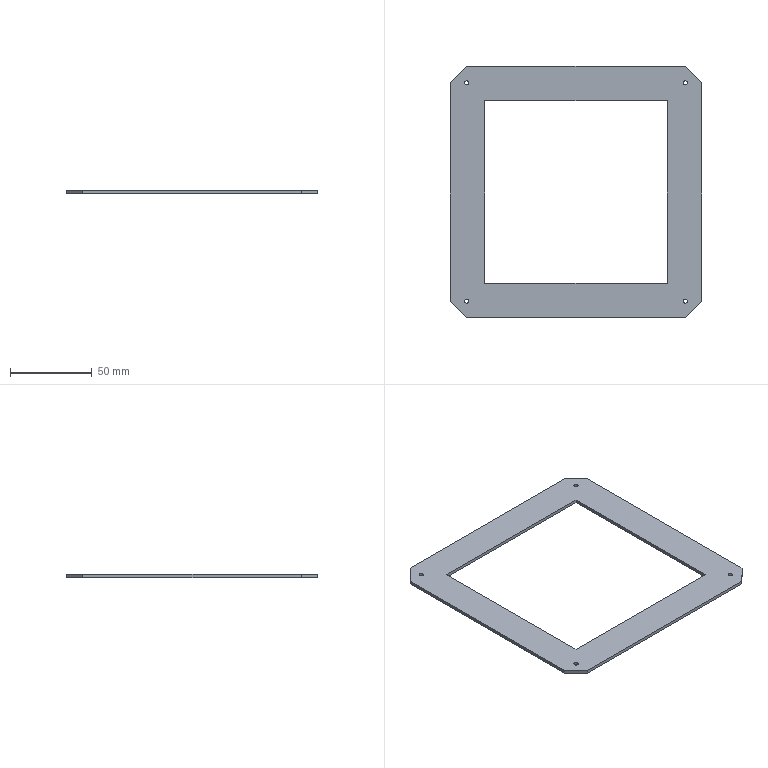Part | STEP file | 11-TG-00111 | 1 solid | 22 faces | box 154 x 154 x 2 mm | volume 21905 mm3 | plane 14 | cylinder 8 | commonest cylinder face diameters 2.5 x8
STEP:
#1=CARTESIAN_POINT('',(8.75,10.,0.));
#2=VERTEX_POINT('',#1);
#3=CARTESIAN_POINT('',(11.25,10.,0.));
#4=VERTEX_POINT('',#3);
#5=CARTESIAN_POINT('',(10.,10.,0.));
#6=DIRECTION('',(0.,0.,1.));
#7=DIRECTION('',(1.,0.,0.));
#8=AXIS2_PLACEMENT_3D('',#5,#6,#7);
#9=CIRCLE('',#8,1.25);
#10=EDGE_CURVE('',#2,#4,#9,.T.);
#11=ORIENTED_EDGE('',*,*,#10,.F.);
#12=CARTESIAN_POINT('',(8.75,10.,2.));
#13=VERTEX_POINT('',#12);
#14=CARTESIAN_POINT('',(8.75,10.,2.));
#15=DIRECTION('',(0.,0.,1.));
#16=VECTOR('',#15,1000.);
#17=LINE('',#14,#16);
#18=EDGE_CURVE('',#2,#13,#17,.T.);
#19=ORIENTED_EDGE('',*,*,#18,.T.);
#20=CARTESIAN_POINT('',(11.25,10.,2.));
#21=VERTEX_POINT('',#20);
#22=CARTESIAN_POINT('',(10.,10.,2.));
#23=DIRECTION('',(0.,0.,1.));
#24=DIRECTION('',(1.,0.,0.));
#25=AXIS2_PLACEMENT_3D('',#22,#23,#24);
#26=CIRCLE('',#25,1.25);
#27=EDGE_CURVE('',#13,#21,#26,.T.);
#28=ORIENTED_EDGE('',*,*,#27,.T.);
#29=CARTESIAN_POINT('',(11.25,10.,2.));
#30=DIRECTION('',(0.,0.,1.));
#31=VECTOR('',#30,1000.);
#32=LINE('',#29,#31);
#33=EDGE_CURVE('',#4,#21,#32,.T.);
#34=ORIENTED_EDGE('',*,*,#33,.F.);
#35=EDGE_LOOP('',(#11,#19,#28,#34));
#36=FACE_OUTER_BOUND('',#35,.T.);
#37=CARTESIAN_POINT('',(10.,10.,2.));
#38=DIRECTION('',(0.,0.,1.));
#39=DIRECTION('',(1.,0.,0.));
#40=AXIS2_PLACEMENT_3D('',#37,#38,#39);
#41=CYLINDRICAL_SURFACE('',#40,1.25);
#42=ADVANCED_FACE('',(#36),#41,.F.);
#43=CARTESIAN_POINT('',(142.75,10.,0.));
#44=VERTEX_POINT('',#43);
#45=CARTESIAN_POINT('',(145.25,10.,0.));
#46=VERTEX_POINT('',#45);
#47=CARTESIAN_POINT('',(144.,10.,0.));
#48=DIRECTION('',(0.,0.,1.));
#49=DIRECTION('',(1.,0.,0.));
#50=AXIS2_PLACEMENT_3D('',#47,#48,#49);
#51=CIRCLE('',#50,1.25);
#52=EDGE_CURVE('',#44,#46,#51,.T.);
#53=ORIENTED_EDGE('',*,*,#52,.F.);
#54=CARTESIAN_POINT('',(142.75,10.,2.));
#55=VERTEX_POINT('',#54);
#56=CARTESIAN_POINT('',(142.75,10.,2.));
#57=DIRECTION('',(0.,0.,1.));
#58=VECTOR('',#57,1000.);
#59=LINE('',#56,#58);
#60=EDGE_CURVE('',#44,#55,#59,.T.);
#61=ORIENTED_EDGE('',*,*,#60,.T.);
#62=CARTESIAN_POINT('',(145.25,10.,2.));
#63=VERTEX_POINT('',#62);
#64=CARTESIAN_POINT('',(144.,10.,2.));
#65=DIRECTION('',(0.,0.,1.));
#66=DIRECTION('',(1.,0.,0.));
#67=AXIS2_PLACEMENT_3D('',#64,#65,#66);
#68=CIRCLE('',#67,1.25);
#69=EDGE_CURVE('',#55,#63,#68,.T.);
#70=ORIENTED_EDGE('',*,*,#69,.T.);
#71=CARTESIAN_POINT('',(145.25,10.,2.));
#72=DIRECTION('',(0.,0.,1.));
#73=VECTOR('',#72,1000.);
#74=LINE('',#71,#73);
#75=EDGE_CURVE('',#46,#63,#74,.T.);
#76=ORIENTED_EDGE('',*,*,#75,.F.);
#77=EDGE_LOOP('',(#53,#61,#70,#76));
#78=FACE_OUTER_BOUND('',#77,.T.);
#79=CARTESIAN_POINT('',(144.,10.,2.));
#80=DIRECTION('',(0.,0.,1.));
#81=DIRECTION('',(1.,0.,0.));
#82=AXIS2_PLACEMENT_3D('',#79,#80,#81);
#83=CYLINDRICAL_SURFACE('',#82,1.25);
#84=ADVANCED_FACE('',(#78),#83,.F.);
#85=CARTESIAN_POINT('',(142.75,144.,0.));
#86=VERTEX_POINT('',#85);
#87=CARTESIAN_POINT('',(145.25,144.,0.));
#88=VERTEX_POINT('',#87);
#89=CARTESIAN_POINT('',(144.,144.,0.));
#90=DIRECTION('',(0.,0.,1.));
#91=DIRECTION('',(1.,0.,0.));
#92=AXIS2_PLACEMENT_3D('',#89,#90,#91);
#93=CIRCLE('',#92,1.25);
#94=EDGE_CURVE('',#86,#88,#93,.T.);
#95=ORIENTED_EDGE('',*,*,#94,.F.);
#96=CARTESIAN_POINT('',(142.75,144.,2.));
#97=VERTEX_POINT('',#96);
#98=CARTESIAN_POINT('',(142.75,144.,2.));
#99=DIRECTION('',(0.,0.,1.));
#100=VECTOR('',#99,1000.);
#101=LINE('',#98,#100);
#102=EDGE_CURVE('',#86,#97,#101,.T.);
#103=ORIENTED_EDGE('',*,*,#102,.T.);
#104=CARTESIAN_POINT('',(145.25,144.,2.));
#105=VERTEX_POINT('',#104);
#106=CARTESIAN_POINT('',(144.,144.,2.));
#107=DIRECTION('',(0.,0.,1.));
#108=DIRECTION('',(1.,0.,0.));
#109=AXIS2_PLACEMENT_3D('',#106,#107,#108);
#110=CIRCLE('',#109,1.25);
#111=EDGE_CURVE('',#97,#105,#110,.T.);
#112=ORIENTED_EDGE('',*,*,#111,.T.);
#113=CARTESIAN_POINT('',(145.25,144.,2.));
#114=DIRECTION('',(0.,0.,1.));
#115=VECTOR('',#114,1000.);
#116=LINE('',#113,#115);
#117=EDGE_CURVE('',#88,#105,#116,.T.);
#118=ORIENTED_EDGE('',*,*,#117,.F.);
#119=EDGE_LOOP('',(#95,#103,#112,#118));
#120=FACE_OUTER_BOUND('',#119,.T.);
#121=CARTESIAN_POINT('',(144.,144.,2.));
#122=DIRECTION('',(0.,0.,1.));
#123=DIRECTION('',(1.,0.,0.));
#124=AXIS2_PLACEMENT_3D('',#121,#122,#123);
#125=CYLINDRICAL_SURFACE('',#124,1.25);
#126=ADVANCED_FACE('',(#120),#125,.F.);
#127=CARTESIAN_POINT('',(8.75,144.,0.));
#128=VERTEX_POINT('',#127);
#129=CARTESIAN_POINT('',(11.25,144.,0.));
#130=VERTEX_POINT('',#129);
#131=CARTESIAN_POINT('',(10.,144.,0.));
#132=DIRECTION('',(0.,0.,1.));
#133=DIRECTION('',(1.,0.,0.));
#134=AXIS2_PLACEMENT_3D('',#131,#132,#133);
#135=CIRCLE('',#134,1.25);
#136=EDGE_CURVE('',#128,#130,#135,.T.);
#137=ORIENTED_EDGE('',*,*,#136,.F.);
#138=CARTESIAN_POINT('',(8.75,144.,2.));
#139=VERTEX_POINT('',#138);
#140=CARTESIAN_POINT('',(8.75,144.,2.));
#141=DIRECTION('',(0.,0.,1.));
#142=VECTOR('',#141,1000.);
#143=LINE('',#140,#142);
#144=EDGE_CURVE('',#128,#139,#143,.T.);
#145=ORIENTED_EDGE('',*,*,#144,.T.);
#146=CARTESIAN_POINT('',(11.25,144.,2.));
#147=VERTEX_POINT('',#146);
#148=CARTESIAN_POINT('',(10.,144.,2.));
#149=DIRECTION('',(0.,0.,1.));
#150=DIRECTION('',(1.,0.,0.));
#151=AXIS2_PLACEMENT_3D('',#148,#149,#150);
#152=CIRCLE('',#151,1.25);
#153=EDGE_CURVE('',#139,#147,#152,.T.);
#154=ORIENTED_EDGE('',*,*,#153,.T.);
#155=CARTESIAN_POINT('',(11.25,144.,2.));
#156=DIRECTION('',(0.,0.,1.));
#157=VECTOR('',#156,1000.);
#158=LINE('',#155,#157);
#159=EDGE_CURVE('',#130,#147,#158,.T.);
#160=ORIENTED_EDGE('',*,*,#159,.F.);
#161=EDGE_LOOP('',(#137,#145,#154,#160));
#162=FACE_OUTER_BOUND('',#161,.T.);
#163=CARTESIAN_POINT('',(10.,144.,2.));
#164=DIRECTION('',(0.,0.,1.));
#165=DIRECTION('',(1.,0.,0.));
#166=AXIS2_PLACEMENT_3D('',#163,#164,#165);
#167=CYLINDRICAL_SURFACE('',#166,1.25);
#168=ADVANCED_FACE('',(#162),#167,.F.);
#169=CARTESIAN_POINT('',(144.,10.,0.));
#170=DIRECTION('',(0.,0.,1.));
#171=DIRECTION('',(1.,0.,0.));
#172=AXIS2_PLACEMENT_3D('',#169,#170,#171);
#173=CIRCLE('',#172,1.25);
#174=EDGE_CURVE('',#46,#44,#173,.T.);
#175=ORIENTED_EDGE('',*,*,#174,.T.);
#176=ORIENTED_EDGE('',*,*,#52,.T.);
#177=EDGE_LOOP('',(#175,#176));
#178=FACE_BOUND('',#177,.T.);
#179=CARTESIAN_POINT('',(10.,144.,0.));
#180=DIRECTION('',(0.,0.,1.));
#181=DIRECTION('',(1.,0.,0.));
#182=AXIS2_PLACEMENT_3D('',#179,#180,#181);
#183=CIRCLE('',#182,1.25);
#184=EDGE_CURVE('',#130,#128,#183,.T.);
#185=ORIENTED_EDGE('',*,*,#184,.T.);
#186=ORIENTED_EDGE('',*,*,#136,.T.);
#187=EDGE_LOOP('',(#185,#186));
#188=FACE_BOUND('',#187,.T.);
#189=CARTESIAN_POINT('',(0.,144.,0.));
#190=VERTEX_POINT('',#189);
#191=CARTESIAN_POINT('',(0.,10.,0.));
#192=VERTEX_POINT('',#191);
#193=CARTESIAN_POINT('',(0.,0.,0.));
#194=DIRECTION('',(0.,-1.,0.));
#195=VECTOR('',#194,1000.);
#196=LINE('',#193,#195);
#197=EDGE_CURVE('',#190,#192,#196,.T.);
#198=ORIENTED_EDGE('',*,*,#197,.F.);
#199=CARTESIAN_POINT('',(10.,154.,0.));
#200=VERTEX_POINT('',#199);
#201=CARTESIAN_POINT('',(-72.,72.,0.));
#202=DIRECTION('',(0.7071,0.7071,0.));
#203=VECTOR('',#202,1000.);
#204=LINE('',#201,#203);
#205=EDGE_CURVE('',#190,#200,#204,.T.);
#206=ORIENTED_EDGE('',*,*,#205,.T.);
#207=CARTESIAN_POINT('',(144.,154.,0.));
#208=VERTEX_POINT('',#207);
#209=CARTESIAN_POINT('',(0.,154.,0.));
#210=DIRECTION('',(-1.,0.,0.));
#211=VECTOR('',#210,1000.);
#212=LINE('',#209,#211);
#213=EDGE_CURVE('',#208,#200,#212,.T.);
#214=ORIENTED_EDGE('',*,*,#213,.F.);
#215=CARTESIAN_POINT('',(154.,144.,0.));
#216=VERTEX_POINT('',#215);
#217=CARTESIAN_POINT('',(149.,149.,0.));
#218=DIRECTION('',(0.7071,-0.7071,0.));
#219=VECTOR('',#218,1000.);
#220=LINE('',#217,#219);
#221=EDGE_CURVE('',#208,#216,#220,.T.);
#222=ORIENTED_EDGE('',*,*,#221,.T.);
#223=CARTESIAN_POINT('',(154.,10.,0.));
#224=VERTEX_POINT('',#223);
#225=CARTESIAN_POINT('',(154.,0.,0.));
#226=DIRECTION('',(0.,1.,0.));
#227=VECTOR('',#226,1000.);
#228=LINE('',#225,#227);
#229=EDGE_CURVE('',#224,#216,#228,.T.);
#230=ORIENTED_EDGE('',*,*,#229,.F.);
#231=CARTESIAN_POINT('',(144.,0.,0.));
#232=VERTEX_POINT('',#231);
#233=CARTESIAN_POINT('',(72.,-72.,0.));
#234=DIRECTION('',(-0.7071,-0.7071,0.));
#235=VECTOR('',#234,1000.);
#236=LINE('',#233,#235);
#237=EDGE_CURVE('',#224,#232,#236,.T.);
#238=ORIENTED_EDGE('',*,*,#237,.T.);
#239=CARTESIAN_POINT('',(10.,0.,0.));
#240=VERTEX_POINT('',#239);
#241=CARTESIAN_POINT('',(0.,0.,0.));
#242=DIRECTION('',(1.,0.,0.));
#243=VECTOR('',#242,1000.);
#244=LINE('',#241,#243);
#245=EDGE_CURVE('',#240,#232,#244,.T.);
#246=ORIENTED_EDGE('',*,*,#245,.F.);
#247=CARTESIAN_POINT('',(5.,5.,0.));
#248=DIRECTION('',(-0.7071,0.7071,0.));
#249=VECTOR('',#248,1000.);
#250=LINE('',#247,#249);
#251=EDGE_CURVE('',#240,#192,#250,.T.);
#252=ORIENTED_EDGE('',*,*,#251,.T.);
#253=EDGE_LOOP('',(#198,#206,#214,#222,#230,#238,#246,#252));
#254=FACE_OUTER_BOUND('',#253,.T.);
#255=CARTESIAN_POINT('',(133.,133.,0.));
#256=VERTEX_POINT('',#255);
#257=CARTESIAN_POINT('',(21.,133.,0.));
#258=VERTEX_POINT('',#257);
#259=CARTESIAN_POINT('',(21.,133.,0.));
#260=DIRECTION('',(-1.,0.,0.));
#261=VECTOR('',#260,1000.);
#262=LINE('',#259,#261);
#263=EDGE_CURVE('',#256,#258,#262,.T.);
#264=ORIENTED_EDGE('',*,*,#263,.T.);
#265=CARTESIAN_POINT('',(21.,21.,0.));
#266=VERTEX_POINT('',#265);
#267=CARTESIAN_POINT('',(21.,21.,0.));
#268=DIRECTION('',(0.,-1.,0.));
#269=VECTOR('',#268,1000.);
#270=LINE('',#267,#269);
#271=EDGE_CURVE('',#258,#266,#270,.T.);
#272=ORIENTED_EDGE('',*,*,#271,.T.);
#273=CARTESIAN_POINT('',(133.,21.,0.));
#274=VERTEX_POINT('',#273);
#275=CARTESIAN_POINT('',(21.,21.,0.));
#276=DIRECTION('',(1.,0.,0.));
#277=VECTOR('',#276,1000.);
#278=LINE('',#275,#277);
#279=EDGE_CURVE('',#266,#274,#278,.T.);
#280=ORIENTED_EDGE('',*,*,#279,.T.);
#281=CARTESIAN_POINT('',(133.,21.,0.));
#282=DIRECTION('',(0.,1.,0.));
#283=VECTOR('',#282,1000.);
#284=LINE('',#281,#283);
#285=EDGE_CURVE('',#274,#256,#284,.T.);
#286=ORIENTED_EDGE('',*,*,#285,.T.);
#287=EDGE_LOOP('',(#264,#272,#280,#286));
#288=FACE_BOUND('',#287,.T.);
#289=CARTESIAN_POINT('',(144.,144.,0.));
#290=DIRECTION('',(0.,0.,1.));
#291=DIRECTION('',(1.,0.,0.));
#292=AXIS2_PLACEMENT_3D('',#289,#290,#291);
#293=CIRCLE('',#292,1.25);
#294=EDGE_CURVE('',#88,#86,#293,.T.);
#295=ORIENTED_EDGE('',*,*,#294,.T.);
#296=ORIENTED_EDGE('',*,*,#94,.T.);
#297=EDGE_LOOP('',(#295,#296));
#298=FACE_BOUND('',#297,.T.);
#299=CARTESIAN_POINT('',(10.,10.,0.));
#300=DIRECTION('',(0.,0.,1.));
#301=DIRECTION('',(1.,0.,0.));
#302=AXIS2_PLACEMENT_3D('',#299,#300,#301);
#303=CIRCLE('',#302,1.25);
#304=EDGE_CURVE('',#4,#2,#303,.T.);
#305=ORIENTED_EDGE('',*,*,#304,.T.);
#306=ORIENTED_EDGE('',*,*,#10,.T.);
#307=EDGE_LOOP('',(#305,#306));
#308=FACE_BOUND('',#307,.T.);
#309=CARTESIAN_POINT('',(0.,0.,0.));
#310=DIRECTION('',(0.,0.,-1.));
#311=DIRECTION('',(-1.,0.,0.));
#312=AXIS2_PLACEMENT_3D('',#309,#310,#311);
#313=PLANE('',#312);
#314=ADVANCED_FACE('',(#178,#188,#254,#288,#298,#308),#313,.T.);
#315=CARTESIAN_POINT('',(144.,10.,2.));
#316=DIRECTION('',(0.,0.,1.));
#317=DIRECTION('',(1.,0.,0.));
#318=AXIS2_PLACEMENT_3D('',#315,#316,#317);
#319=CIRCLE('',#318,1.25);
#320=EDGE_CURVE('',#63,#55,#319,.T.);
#321=ORIENTED_EDGE('',*,*,#320,.F.);
#322=ORIENTED_EDGE('',*,*,#69,.F.);
#323=EDGE_LOOP('',(#321,#322));
#324=FACE_BOUND('',#323,.T.);
#325=CARTESIAN_POINT('',(10.,144.,2.));
#326=DIRECTION('',(0.,0.,1.));
#327=DIRECTION('',(1.,0.,0.));
#328=AXIS2_PLACEMENT_3D('',#325,#326,#327);
#329=CIRCLE('',#328,1.25);
#330=EDGE_CURVE('',#147,#139,#329,.T.);
#331=ORIENTED_EDGE('',*,*,#330,.F.);
#332=ORIENTED_EDGE('',*,*,#153,.F.);
#333=EDGE_LOOP('',(#331,#332));
#334=FACE_BOUND('',#333,.T.);
#335=CARTESIAN_POINT('',(144.,154.,2.));
#336=VERTEX_POINT('',#335);
#337=CARTESIAN_POINT('',(10.,154.,2.));
#338=VERTEX_POINT('',#337);
#339=CARTESIAN_POINT('',(0.,154.,2.));
#340=DIRECTION('',(-1.,0.,0.));
#341=VECTOR('',#340,1000.);
#342=LINE('',#339,#341);
#343=EDGE_CURVE('',#336,#338,#342,.T.);
#344=ORIENTED_EDGE('',*,*,#343,.T.);
#345=CARTESIAN_POINT('',(0.,144.,2.));
#346=VERTEX_POINT('',#345);
#347=CARTESIAN_POINT('',(0.,144.,2.));
#348=DIRECTION('',(-0.7071,-0.7071,0.));
#349=VECTOR('',#348,1000.);
#350=LINE('',#347,#349);
#351=EDGE_CURVE('',#338,#346,#350,.T.);
#352=ORIENTED_EDGE('',*,*,#351,.T.);
#353=CARTESIAN_POINT('',(0.,10.,2.));
#354=VERTEX_POINT('',#353);
#355=CARTESIAN_POINT('',(0.,0.,2.));
#356=DIRECTION('',(0.,-1.,0.));
#357=VECTOR('',#356,1000.);
#358=LINE('',#355,#357);
#359=EDGE_CURVE('',#346,#354,#358,.T.);
#360=ORIENTED_EDGE('',*,*,#359,.T.);
#361=CARTESIAN_POINT('',(10.,0.,2.));
#362=VERTEX_POINT('',#361);
#363=CARTESIAN_POINT('',(10.,0.,2.));
#364=DIRECTION('',(0.7071,-0.7071,0.));
#365=VECTOR('',#364,1000.);
#366=LINE('',#363,#365);
#367=EDGE_CURVE('',#354,#362,#366,.T.);
#368=ORIENTED_EDGE('',*,*,#367,.T.);
#369=CARTESIAN_POINT('',(144.,0.,2.));
#370=VERTEX_POINT('',#369);
#371=CARTESIAN_POINT('',(0.,0.,2.));
#372=DIRECTION('',(1.,0.,0.));
#373=VECTOR('',#372,1000.);
#374=LINE('',#371,#373);
#375=EDGE_CURVE('',#362,#370,#374,.T.);
#376=ORIENTED_EDGE('',*,*,#375,.T.);
#377=CARTESIAN_POINT('',(154.,10.,2.));
#378=VERTEX_POINT('',#377);
#379=CARTESIAN_POINT('',(154.,10.,2.));
#380=DIRECTION('',(0.7071,0.7071,0.));
#381=VECTOR('',#380,1000.);
#382=LINE('',#379,#381);
#383=EDGE_CURVE('',#370,#378,#382,.T.);
#384=ORIENTED_EDGE('',*,*,#383,.T.);
#385=CARTESIAN_POINT('',(154.,144.,2.));
#386=VERTEX_POINT('',#385);
#387=CARTESIAN_POINT('',(154.,0.,2.));
#388=DIRECTION('',(0.,1.,0.));
#389=VECTOR('',#388,1000.);
#390=LINE('',#387,#389);
#391=EDGE_CURVE('',#378,#386,#390,.T.);
#392=ORIENTED_EDGE('',*,*,#391,.T.);
#393=CARTESIAN_POINT('',(144.,154.,2.));
#394=DIRECTION('',(-0.7071,0.7071,0.));
#395=VECTOR('',#394,1000.);
#396=LINE('',#393,#395);
#397=EDGE_CURVE('',#386,#336,#396,.T.);
#398=ORIENTED_EDGE('',*,*,#397,.T.);
#399=EDGE_LOOP('',(#344,#352,#360,#368,#376,#384,#392,#398));
#400=FACE_OUTER_BOUND('',#399,.T.);
#401=CARTESIAN_POINT('',(21.,133.,2.));
#402=VERTEX_POINT('',#401);
#403=CARTESIAN_POINT('',(21.,21.,2.));
#404=VERTEX_POINT('',#403);
#405=CARTESIAN_POINT('',(21.,21.,2.));
#406=DIRECTION('',(0.,-1.,0.));
#407=VECTOR('',#406,1000.);
#408=LINE('',#405,#407);
#409=EDGE_CURVE('',#402,#404,#408,.T.);
#410=ORIENTED_EDGE('',*,*,#409,.F.);
#411=CARTESIAN_POINT('',(133.,133.,2.));
#412=VERTEX_POINT('',#411);
#413=CARTESIAN_POINT('',(21.,133.,2.));
#414=DIRECTION('',(-1.,0.,0.));
#415=VECTOR('',#414,1000.);
#416=LINE('',#413,#415);
#417=EDGE_CURVE('',#412,#402,#416,.T.);
#418=ORIENTED_EDGE('',*,*,#417,.F.);
#419=CARTESIAN_POINT('',(133.,21.,2.));
#420=VERTEX_POINT('',#419);
#421=CARTESIAN_POINT('',(133.,21.,2.));
#422=DIRECTION('',(0.,1.,0.));
#423=VECTOR('',#422,1000.);
#424=LINE('',#421,#423);
#425=EDGE_CURVE('',#420,#412,#424,.T.);
#426=ORIENTED_EDGE('',*,*,#425,.F.);
#427=CARTESIAN_POINT('',(21.,21.,2.));
#428=DIRECTION('',(1.,0.,0.));
#429=VECTOR('',#428,1000.);
#430=LINE('',#427,#429);
#431=EDGE_CURVE('',#404,#420,#430,.T.);
#432=ORIENTED_EDGE('',*,*,#431,.F.);
#433=EDGE_LOOP('',(#410,#418,#426,#432));
#434=FACE_BOUND('',#433,.T.);
#435=CARTESIAN_POINT('',(144.,144.,2.));
#436=DIRECTION('',(0.,0.,1.));
#437=DIRECTION('',(1.,0.,0.));
#438=AXIS2_PLACEMENT_3D('',#435,#436,#437);
#439=CIRCLE('',#438,1.25);
#440=EDGE_CURVE('',#105,#97,#439,.T.);
#441=ORIENTED_EDGE('',*,*,#440,.F.);
#442=ORIENTED_EDGE('',*,*,#111,.F.);
#443=EDGE_LOOP('',(#441,#442));
#444=FACE_BOUND('',#443,.T.);
#445=CARTESIAN_POINT('',(10.,10.,2.));
#446=DIRECTION('',(0.,0.,1.));
#447=DIRECTION('',(1.,0.,0.));
#448=AXIS2_PLACEMENT_3D('',#445,#446,#447);
#449=CIRCLE('',#448,1.25);
#450=EDGE_CURVE('',#21,#13,#449,.T.);
#451=ORIENTED_EDGE('',*,*,#450,.F.);
#452=ORIENTED_EDGE('',*,*,#27,.F.);
#453=EDGE_LOOP('',(#451,#452));
#454=FACE_BOUND('',#453,.T.);
#455=CARTESIAN_POINT('',(0.,0.,2.));
#456=DIRECTION('',(0.,0.,-1.));
#457=DIRECTION('',(-1.,0.,0.));
#458=AXIS2_PLACEMENT_3D('',#455,#456,#457);
#459=PLANE('',#458);
#460=ADVANCED_FACE('',(#324,#334,#400,#434,#444,#454),#459,.F.);
#461=ORIENTED_EDGE('',*,*,#359,.F.);
#462=CARTESIAN_POINT('',(0.,144.,2.));
#463=DIRECTION('',(0.,0.,-1.));
#464=VECTOR('',#463,1000.);
#465=LINE('',#462,#464);
#466=EDGE_CURVE('',#346,#190,#465,.T.);
#467=ORIENTED_EDGE('',*,*,#466,.T.);
#468=ORIENTED_EDGE('',*,*,#197,.T.);
#469=CARTESIAN_POINT('',(0.,10.,2.));
#470=DIRECTION('',(0.,0.,1.));
#471=VECTOR('',#470,1000.);
#472=LINE('',#469,#471);
#473=EDGE_CURVE('',#192,#354,#472,.T.);
#474=ORIENTED_EDGE('',*,*,#473,.T.);
#475=EDGE_LOOP('',(#461,#467,#468,#474));
#476=FACE_OUTER_BOUND('',#475,.T.);
#477=CARTESIAN_POINT('',(0.,0.,2.));
#478=DIRECTION('',(1.,0.,0.));
#479=DIRECTION('',(0.,0.,-1.));
#480=AXIS2_PLACEMENT_3D('',#477,#478,#479);
#481=PLANE('',#480);
#482=ADVANCED_FACE('',(#476),#481,.F.);
#483=ORIENTED_EDGE('',*,*,#245,.T.);
#484=CARTESIAN_POINT('',(144.,0.,2.));
#485=DIRECTION('',(0.,0.,1.));
#486=VECTOR('',#485,1000.);
#487=LINE('',#484,#486);
#488=EDGE_CURVE('',#232,#370,#487,.T.);
#489=ORIENTED_EDGE('',*,*,#488,.T.);
#490=ORIENTED_EDGE('',*,*,#375,.F.);
#491=CARTESIAN_POINT('',(10.,0.,2.));
#492=DIRECTION('',(0.,0.,-1.));
#493=VECTOR('',#492,1000.);
#494=LINE('',#491,#493);
#495=EDGE_CURVE('',#362,#240,#494,.T.);
#496=ORIENTED_EDGE('',*,*,#495,.T.);
#497=EDGE_LOOP('',(#483,#489,#490,#496));
#498=FACE_OUTER_BOUND('',#497,.T.);
#499=CARTESIAN_POINT('',(0.,0.,2.));
#500=DIRECTION('',(0.,1.,0.));
#501=DIRECTION('',(0.,0.,1.));
#502=AXIS2_PLACEMENT_3D('',#499,#500,#501);
#503=PLANE('',#502);
#504=ADVANCED_FACE('',(#498),#503,.F.);
#505=ORIENTED_EDGE('',*,*,#391,.F.);
#506=CARTESIAN_POINT('',(154.,10.,2.));
#507=DIRECTION('',(0.,0.,-1.));
#508=VECTOR('',#507,1000.);
#509=LINE('',#506,#508);
#510=EDGE_CURVE('',#378,#224,#509,.T.);
#511=ORIENTED_EDGE('',*,*,#510,.T.);
#512=ORIENTED_EDGE('',*,*,#229,.T.);
#513=CARTESIAN_POINT('',(154.,144.,2.));
#514=DIRECTION('',(0.,0.,1.));
#515=VECTOR('',#514,1000.);
#516=LINE('',#513,#515);
#517=EDGE_CURVE('',#216,#386,#516,.T.);
#518=ORIENTED_EDGE('',*,*,#517,.T.);
#519=EDGE_LOOP('',(#505,#511,#512,#518));
#520=FACE_OUTER_BOUND('',#519,.T.);
#521=CARTESIAN_POINT('',(154.,0.,2.));
#522=DIRECTION('',(-1.,0.,0.));
#523=DIRECTION('',(0.,0.,1.));
#524=AXIS2_PLACEMENT_3D('',#521,#522,#523);
#525=PLANE('',#524);
#526=ADVANCED_FACE('',(#520),#525,.F.);
#527=ORIENTED_EDGE('',*,*,#213,.T.);
#528=CARTESIAN_POINT('',(10.,154.,2.));
#529=DIRECTION('',(0.,0.,1.));
#530=VECTOR('',#529,1000.);
#531=LINE('',#528,#530);
#532=EDGE_CURVE('',#200,#338,#531,.T.);
#533=ORIENTED_EDGE('',*,*,#532,.T.);
#534=ORIENTED_EDGE('',*,*,#343,.F.);
#535=CARTESIAN_POINT('',(144.,154.,2.));
#536=DIRECTION('',(0.,0.,-1.));
#537=VECTOR('',#536,1000.);
#538=LINE('',#535,#537);
#539=EDGE_CURVE('',#336,#208,#538,.T.);
#540=ORIENTED_EDGE('',*,*,#539,.T.);
#541=EDGE_LOOP('',(#527,#533,#534,#540));
#542=FACE_OUTER_BOUND('',#541,.T.);
#543=CARTESIAN_POINT('',(0.,154.,2.));
#544=DIRECTION('',(0.,-1.,0.));
#545=DIRECTION('',(0.,0.,-1.));
#546=AXIS2_PLACEMENT_3D('',#543,#544,#545);
#547=PLANE('',#546);
#548=ADVANCED_FACE('',(#542),#547,.F.);
#549=ORIENTED_EDGE('',*,*,#271,.F.);
#550=CARTESIAN_POINT('',(21.,133.,2.));
#551=DIRECTION('',(0.,0.,-1.));
#552=VECTOR('',#551,1000.);
#553=LINE('',#550,#552);
#554=EDGE_CURVE('',#402,#258,#553,.T.);
#555=ORIENTED_EDGE('',*,*,#554,.F.);
#556=ORIENTED_EDGE('',*,*,#409,.T.);
#557=CARTESIAN_POINT('',(21.,21.,2.));
#558=DIRECTION('',(0.,0.,-1.));
#559=VECTOR('',#558,1000.);
#560=LINE('',#557,#559);
#561=EDGE_CURVE('',#404,#266,#560,.T.);
#562=ORIENTED_EDGE('',*,*,#561,.T.);
#563=EDGE_LOOP('',(#549,#555,#556,#562));
#564=FACE_OUTER_BOUND('',#563,.T.);
#565=CARTESIAN_POINT('',(21.,21.,2.));
#566=DIRECTION('',(1.,0.,0.));
#567=DIRECTION('',(0.,0.,-1.));
#568=AXIS2_PLACEMENT_3D('',#565,#566,#567);
#569=PLANE('',#568);
#570=ADVANCED_FACE('',(#564),#569,.T.);
#571=ORIENTED_EDGE('',*,*,#279,.F.);
#572=ORIENTED_EDGE('',*,*,#561,.F.);
#573=ORIENTED_EDGE('',*,*,#431,.T.);
#574=CARTESIAN_POINT('',(133.,21.,2.));
#575=DIRECTION('',(0.,0.,-1.));
#576=VECTOR('',#575,1000.);
#577=LINE('',#574,#576);
#578=EDGE_CURVE('',#420,#274,#577,.T.);
#579=ORIENTED_EDGE('',*,*,#578,.T.);
#580=EDGE_LOOP('',(#571,#572,#573,#579));
#581=FACE_OUTER_BOUND('',#580,.T.);
#582=CARTESIAN_POINT('',(21.,21.,2.));
#583=DIRECTION('',(0.,1.,0.));
#584=DIRECTION('',(0.,0.,1.));
#585=AXIS2_PLACEMENT_3D('',#582,#583,#584);
#586=PLANE('',#585);
#587=ADVANCED_FACE('',(#581),#586,.T.);
#588=ORIENTED_EDGE('',*,*,#285,.F.);
#589=ORIENTED_EDGE('',*,*,#578,.F.);
#590=ORIENTED_EDGE('',*,*,#425,.T.);
#591=CARTESIAN_POINT('',(133.,133.,2.));
#592=DIRECTION('',(0.,0.,-1.));
#593=VECTOR('',#592,1000.);
#594=LINE('',#591,#593);
#595=EDGE_CURVE('',#412,#256,#594,.T.);
#596=ORIENTED_EDGE('',*,*,#595,.T.);
#597=EDGE_LOOP('',(#588,#589,#590,#596));
#598=FACE_OUTER_BOUND('',#597,.T.);
#599=CARTESIAN_POINT('',(133.,21.,2.));
#600=DIRECTION('',(-1.,0.,0.));
#601=DIRECTION('',(0.,0.,1.));
#602=AXIS2_PLACEMENT_3D('',#599,#600,#601);
#603=PLANE('',#602);
#604=ADVANCED_FACE('',(#598),#603,.T.);
#605=ORIENTED_EDGE('',*,*,#263,.F.);
#606=ORIENTED_EDGE('',*,*,#595,.F.);
#607=ORIENTED_EDGE('',*,*,#417,.T.);
#608=ORIENTED_EDGE('',*,*,#554,.T.);
#609=EDGE_LOOP('',(#605,#606,#607,#608));
#610=FACE_OUTER_BOUND('',#609,.T.);
#611=CARTESIAN_POINT('',(21.,133.,2.));
#612=DIRECTION('',(0.,-1.,0.));
#613=DIRECTION('',(0.,0.,-1.));
#614=AXIS2_PLACEMENT_3D('',#611,#612,#613);
#615=PLANE('',#614);
#616=ADVANCED_FACE('',(#610),#615,.T.);
#617=ORIENTED_EDGE('',*,*,#351,.F.);
#618=ORIENTED_EDGE('',*,*,#532,.F.);
#619=ORIENTED_EDGE('',*,*,#205,.F.);
#620=ORIENTED_EDGE('',*,*,#466,.F.);
#621=EDGE_LOOP('',(#617,#618,#619,#620));
#622=FACE_OUTER_BOUND('',#621,.T.);
#623=CARTESIAN_POINT('',(0.,144.,2.));
#624=DIRECTION('',(0.7071,-0.7071,0.));
#625=DIRECTION('',(0.,0.,-1.));
#626=AXIS2_PLACEMENT_3D('',#623,#624,#625);
#627=PLANE('',#626);
#628=ADVANCED_FACE('',(#622),#627,.F.);
#629=ORIENTED_EDGE('',*,*,#383,.F.);
#630=ORIENTED_EDGE('',*,*,#488,.F.);
#631=ORIENTED_EDGE('',*,*,#237,.F.);
#632=ORIENTED_EDGE('',*,*,#510,.F.);
#633=EDGE_LOOP('',(#629,#630,#631,#632));
#634=FACE_OUTER_BOUND('',#633,.T.);
#635=CARTESIAN_POINT('',(154.,10.,2.));
#636=DIRECTION('',(-0.7071,0.7071,0.));
#637=DIRECTION('',(0.,0.,-1.));
#638=AXIS2_PLACEMENT_3D('',#635,#636,#637);
#639=PLANE('',#638);
#640=ADVANCED_FACE('',(#634),#639,.F.);
#641=ORIENTED_EDGE('',*,*,#367,.F.);
#642=ORIENTED_EDGE('',*,*,#473,.F.);
#643=ORIENTED_EDGE('',*,*,#251,.F.);
#644=ORIENTED_EDGE('',*,*,#495,.F.);
#645=EDGE_LOOP('',(#641,#642,#643,#644));
#646=FACE_OUTER_BOUND('',#645,.T.);
#647=CARTESIAN_POINT('',(10.,0.,2.));
#648=DIRECTION('',(0.7071,0.7071,0.));
#649=DIRECTION('',(0.,0.,-1.));
#650=AXIS2_PLACEMENT_3D('',#647,#648,#649);
#651=PLANE('',#650);
#652=ADVANCED_FACE('',(#646),#651,.F.);
#653=ORIENTED_EDGE('',*,*,#397,.F.);
#654=ORIENTED_EDGE('',*,*,#517,.F.);
#655=ORIENTED_EDGE('',*,*,#221,.F.);
#656=ORIENTED_EDGE('',*,*,#539,.F.);
#657=EDGE_LOOP('',(#653,#654,#655,#656));
#658=FACE_OUTER_BOUND('',#657,.T.);
#659=CARTESIAN_POINT('',(144.,154.,2.));
#660=DIRECTION('',(-0.7071,-0.7071,0.));
#661=DIRECTION('',(0.,0.,-1.));
#662=AXIS2_PLACEMENT_3D('',#659,#660,#661);
#663=PLANE('',#662);
#664=ADVANCED_FACE('',(#658),#663,.F.);
#665=ORIENTED_EDGE('',*,*,#144,.F.);
#666=ORIENTED_EDGE('',*,*,#184,.F.);
#667=ORIENTED_EDGE('',*,*,#159,.T.);
#668=ORIENTED_EDGE('',*,*,#330,.T.);
#669=EDGE_LOOP('',(#665,#666,#667,#668));
#670=FACE_OUTER_BOUND('',#669,.T.);
#671=CARTESIAN_POINT('',(10.,144.,2.));
#672=DIRECTION('',(0.,0.,1.));
#673=DIRECTION('',(1.,0.,0.));
#674=AXIS2_PLACEMENT_3D('',#671,#672,#673);
#675=CYLINDRICAL_SURFACE('',#674,1.25);
#676=ADVANCED_FACE('',(#670),#675,.F.);
#677=ORIENTED_EDGE('',*,*,#102,.F.);
#678=ORIENTED_EDGE('',*,*,#294,.F.);
#679=ORIENTED_EDGE('',*,*,#117,.T.);
#680=ORIENTED_EDGE('',*,*,#440,.T.);
#681=EDGE_LOOP('',(#677,#678,#679,#680));
#682=FACE_OUTER_BOUND('',#681,.T.);
#683=CARTESIAN_POINT('',(144.,144.,2.));
#684=DIRECTION('',(0.,0.,1.));
#685=DIRECTION('',(1.,0.,0.));
#686=AXIS2_PLACEMENT_3D('',#683,#684,#685);
#687=CYLINDRICAL_SURFACE('',#686,1.25);
#688=ADVANCED_FACE('',(#682),#687,.F.);
#689=ORIENTED_EDGE('',*,*,#60,.F.);
#690=ORIENTED_EDGE('',*,*,#174,.F.);
#691=ORIENTED_EDGE('',*,*,#75,.T.);
#692=ORIENTED_EDGE('',*,*,#320,.T.);
#693=EDGE_LOOP('',(#689,#690,#691,#692));
#694=FACE_OUTER_BOUND('',#693,.T.);
#695=CARTESIAN_POINT('',(144.,10.,2.));
#696=DIRECTION('',(0.,0.,1.));
#697=DIRECTION('',(1.,0.,0.));
#698=AXIS2_PLACEMENT_3D('',#695,#696,#697);
#699=CYLINDRICAL_SURFACE('',#698,1.25);
#700=ADVANCED_FACE('',(#694),#699,.F.);
#701=ORIENTED_EDGE('',*,*,#18,.F.);
#702=ORIENTED_EDGE('',*,*,#304,.F.);
#703=ORIENTED_EDGE('',*,*,#33,.T.);
#704=ORIENTED_EDGE('',*,*,#450,.T.);
#705=EDGE_LOOP('',(#701,#702,#703,#704));
#706=FACE_OUTER_BOUND('',#705,.T.);
#707=CARTESIAN_POINT('',(10.,10.,2.));
#708=DIRECTION('',(0.,0.,1.));
#709=DIRECTION('',(1.,0.,0.));
#710=AXIS2_PLACEMENT_3D('',#707,#708,#709);
#711=CYLINDRICAL_SURFACE('',#710,1.25);
#712=ADVANCED_FACE('',(#706),#711,.F.);
#713=CLOSED_SHELL('',(#42,#84,#126,#168,#314,#460,#482,#504,#526,#548,#570,#587,#604,#616,#628,#640,#652,#664,#676,#688,#700,#712));
#714=MANIFOLD_SOLID_BREP('',#713);
#715=CARTESIAN_POINT('',(0.,0.,0.));
#716=DIRECTION('',(0.,0.,1.));
#717=DIRECTION('',(1.,0.,0.));
#718=AXIS2_PLACEMENT_3D('',#715,#716,#717);
#719=(LENGTH_UNIT()NAMED_UNIT(*)SI_UNIT(.MILLI.,.METRE.));
#720=UNCERTAINTY_MEASURE_WITH_UNIT(LENGTH_MEASURE(0.00001),#719,'','');
#721=(NAMED_UNIT(*)PLANE_ANGLE_UNIT()SI_UNIT($,.RADIAN.));
#722=(NAMED_UNIT(*)SI_UNIT($,.STERADIAN.)SOLID_ANGLE_UNIT());
#723=(GEOMETRIC_REPRESENTATION_CONTEXT(3)GLOBAL_UNCERTAINTY_ASSIGNED_CONTEXT((#720))GLOBAL_UNIT_ASSIGNED_CONTEXT((#719,#721,#722))REPRESENTATION_CONTEXT('',''));
#724=ADVANCED_BREP_SHAPE_REPRESENTATION('',(#714,#718),#723);